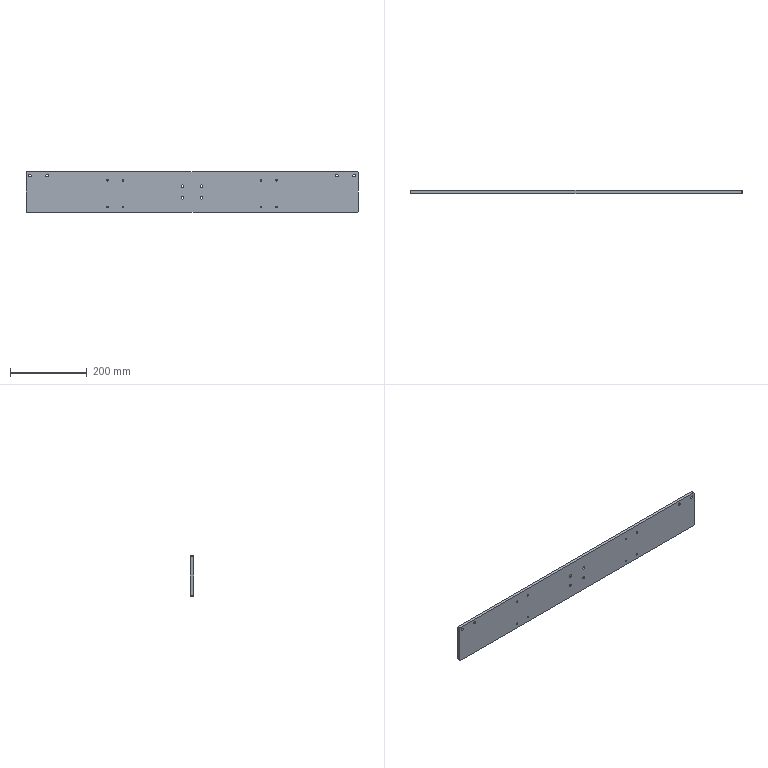Part | SolidWorks | features HoleWzd 3, Chamfer 1, Extrusion 1 | 1 solid | 42 faces | box 865 x 8 x 105 mm | volume 723256 mm3 | cylinder 32 | plane 10 | commonest cylinder face diameters 4.2 x16 6.8 x8 7 x8
STEP:
#1=CARTESIAN_POINT('',(422.5,-4.,39.1));
#2=VERTEX_POINT('',#1);
#3=CARTESIAN_POINT('',(422.5,-4.,45.9));
#4=VERTEX_POINT('',#3);
#5=CARTESIAN_POINT('',(422.5,-4.,42.5));
#6=DIRECTION('',(0.,1.,0.));
#7=DIRECTION('',(0.,0.,1.));
#8=AXIS2_PLACEMENT_3D('',#5,#6,#7);
#9=CIRCLE('',#8,3.4);
#10=EDGE_CURVE('',#2,#4,#9,.T.);
#11=ORIENTED_EDGE('',*,*,#10,.F.);
#12=CARTESIAN_POINT('',(422.5,4.,39.1));
#13=VERTEX_POINT('',#12);
#14=CARTESIAN_POINT('',(422.5,4.,39.1));
#15=DIRECTION('',(0.,1.,0.));
#16=VECTOR('',#15,1000.);
#17=LINE('',#14,#16);
#18=EDGE_CURVE('',#2,#13,#17,.T.);
#19=ORIENTED_EDGE('',*,*,#18,.T.);
#20=CARTESIAN_POINT('',(422.5,4.,45.9));
#21=VERTEX_POINT('',#20);
#22=CARTESIAN_POINT('',(422.5,4.,42.5));
#23=DIRECTION('',(0.,1.,0.));
#24=DIRECTION('',(0.,0.,1.));
#25=AXIS2_PLACEMENT_3D('',#22,#23,#24);
#26=CIRCLE('',#25,3.4);
#27=EDGE_CURVE('',#13,#21,#26,.T.);
#28=ORIENTED_EDGE('',*,*,#27,.T.);
#29=CARTESIAN_POINT('',(422.5,4.,45.9));
#30=DIRECTION('',(0.,1.,0.));
#31=VECTOR('',#30,1000.);
#32=LINE('',#29,#31);
#33=EDGE_CURVE('',#4,#21,#32,.T.);
#34=ORIENTED_EDGE('',*,*,#33,.F.);
#35=EDGE_LOOP('',(#11,#19,#28,#34));
#36=FACE_OUTER_BOUND('',#35,.T.);
#37=CARTESIAN_POINT('',(422.5,4.,42.5));
#38=DIRECTION('',(0.,1.,0.));
#39=DIRECTION('',(0.,0.,1.));
#40=AXIS2_PLACEMENT_3D('',#37,#38,#39);
#41=CYLINDRICAL_SURFACE('',#40,3.4);
#42=ADVANCED_FACE('',(#36),#41,.F.);
#43=CARTESIAN_POINT('',(377.5,-4.,39.1));
#44=VERTEX_POINT('',#43);
#45=CARTESIAN_POINT('',(377.5,-4.,45.9));
#46=VERTEX_POINT('',#45);
#47=CARTESIAN_POINT('',(377.5,-4.,42.5));
#48=DIRECTION('',(0.,1.,0.));
#49=DIRECTION('',(0.,0.,1.));
#50=AXIS2_PLACEMENT_3D('',#47,#48,#49);
#51=CIRCLE('',#50,3.4);
#52=EDGE_CURVE('',#44,#46,#51,.T.);
#53=ORIENTED_EDGE('',*,*,#52,.F.);
#54=CARTESIAN_POINT('',(377.5,4.,39.1));
#55=VERTEX_POINT('',#54);
#56=CARTESIAN_POINT('',(377.5,4.,39.1));
#57=DIRECTION('',(0.,1.,0.));
#58=VECTOR('',#57,1000.);
#59=LINE('',#56,#58);
#60=EDGE_CURVE('',#44,#55,#59,.T.);
#61=ORIENTED_EDGE('',*,*,#60,.T.);
#62=CARTESIAN_POINT('',(377.5,4.,45.9));
#63=VERTEX_POINT('',#62);
#64=CARTESIAN_POINT('',(377.5,4.,42.5));
#65=DIRECTION('',(0.,1.,0.));
#66=DIRECTION('',(0.,0.,1.));
#67=AXIS2_PLACEMENT_3D('',#64,#65,#66);
#68=CIRCLE('',#67,3.4);
#69=EDGE_CURVE('',#55,#63,#68,.T.);
#70=ORIENTED_EDGE('',*,*,#69,.T.);
#71=CARTESIAN_POINT('',(377.5,4.,45.9));
#72=DIRECTION('',(0.,1.,0.));
#73=VECTOR('',#72,1000.);
#74=LINE('',#71,#73);
#75=EDGE_CURVE('',#46,#63,#74,.T.);
#76=ORIENTED_EDGE('',*,*,#75,.F.);
#77=EDGE_LOOP('',(#53,#61,#70,#76));
#78=FACE_OUTER_BOUND('',#77,.T.);
#79=CARTESIAN_POINT('',(377.5,4.,42.5));
#80=DIRECTION('',(0.,1.,0.));
#81=DIRECTION('',(0.,0.,1.));
#82=AXIS2_PLACEMENT_3D('',#79,#80,#81);
#83=CYLINDRICAL_SURFACE('',#82,3.4);
#84=ADVANCED_FACE('',(#78),#83,.F.);
#85=CARTESIAN_POINT('',(-377.5,-4.,39.1));
#86=VERTEX_POINT('',#85);
#87=CARTESIAN_POINT('',(-377.5,-4.,45.9));
#88=VERTEX_POINT('',#87);
#89=CARTESIAN_POINT('',(-377.5,-4.,42.5));
#90=DIRECTION('',(0.,1.,0.));
#91=DIRECTION('',(0.,0.,1.));
#92=AXIS2_PLACEMENT_3D('',#89,#90,#91);
#93=CIRCLE('',#92,3.4);
#94=EDGE_CURVE('',#86,#88,#93,.T.);
#95=ORIENTED_EDGE('',*,*,#94,.F.);
#96=CARTESIAN_POINT('',(-377.5,4.,39.1));
#97=VERTEX_POINT('',#96);
#98=CARTESIAN_POINT('',(-377.5,4.,39.1));
#99=DIRECTION('',(0.,1.,0.));
#100=VECTOR('',#99,1000.);
#101=LINE('',#98,#100);
#102=EDGE_CURVE('',#86,#97,#101,.T.);
#103=ORIENTED_EDGE('',*,*,#102,.T.);
#104=CARTESIAN_POINT('',(-377.5,4.,45.9));
#105=VERTEX_POINT('',#104);
#106=CARTESIAN_POINT('',(-377.5,4.,42.5));
#107=DIRECTION('',(0.,1.,0.));
#108=DIRECTION('',(0.,0.,1.));
#109=AXIS2_PLACEMENT_3D('',#106,#107,#108);
#110=CIRCLE('',#109,3.4);
#111=EDGE_CURVE('',#97,#105,#110,.T.);
#112=ORIENTED_EDGE('',*,*,#111,.T.);
#113=CARTESIAN_POINT('',(-377.5,4.,45.9));
#114=DIRECTION('',(0.,1.,0.));
#115=VECTOR('',#114,1000.);
#116=LINE('',#113,#115);
#117=EDGE_CURVE('',#88,#105,#116,.T.);
#118=ORIENTED_EDGE('',*,*,#117,.F.);
#119=EDGE_LOOP('',(#95,#103,#112,#118));
#120=FACE_OUTER_BOUND('',#119,.T.);
#121=CARTESIAN_POINT('',(-377.5,4.,42.5));
#122=DIRECTION('',(0.,1.,0.));
#123=DIRECTION('',(0.,0.,1.));
#124=AXIS2_PLACEMENT_3D('',#121,#122,#123);
#125=CYLINDRICAL_SURFACE('',#124,3.4);
#126=ADVANCED_FACE('',(#120),#125,.F.);
#127=CARTESIAN_POINT('',(-422.5,-4.,39.1));
#128=VERTEX_POINT('',#127);
#129=CARTESIAN_POINT('',(-422.5,-4.,45.9));
#130=VERTEX_POINT('',#129);
#131=CARTESIAN_POINT('',(-422.5,-4.,42.5));
#132=DIRECTION('',(0.,1.,0.));
#133=DIRECTION('',(0.,0.,1.));
#134=AXIS2_PLACEMENT_3D('',#131,#132,#133);
#135=CIRCLE('',#134,3.4);
#136=EDGE_CURVE('',#128,#130,#135,.T.);
#137=ORIENTED_EDGE('',*,*,#136,.F.);
#138=CARTESIAN_POINT('',(-422.5,4.,39.1));
#139=VERTEX_POINT('',#138);
#140=CARTESIAN_POINT('',(-422.5,4.,39.1));
#141=DIRECTION('',(0.,1.,0.));
#142=VECTOR('',#141,1000.);
#143=LINE('',#140,#142);
#144=EDGE_CURVE('',#128,#139,#143,.T.);
#145=ORIENTED_EDGE('',*,*,#144,.T.);
#146=CARTESIAN_POINT('',(-422.5,4.,45.9));
#147=VERTEX_POINT('',#146);
#148=CARTESIAN_POINT('',(-422.5,4.,42.5));
#149=DIRECTION('',(0.,1.,0.));
#150=DIRECTION('',(0.,0.,1.));
#151=AXIS2_PLACEMENT_3D('',#148,#149,#150);
#152=CIRCLE('',#151,3.4);
#153=EDGE_CURVE('',#139,#147,#152,.T.);
#154=ORIENTED_EDGE('',*,*,#153,.T.);
#155=CARTESIAN_POINT('',(-422.5,4.,45.9));
#156=DIRECTION('',(0.,1.,0.));
#157=VECTOR('',#156,1000.);
#158=LINE('',#155,#157);
#159=EDGE_CURVE('',#130,#147,#158,.T.);
#160=ORIENTED_EDGE('',*,*,#159,.F.);
#161=EDGE_LOOP('',(#137,#145,#154,#160));
#162=FACE_OUTER_BOUND('',#161,.T.);
#163=CARTESIAN_POINT('',(-422.5,4.,42.5));
#164=DIRECTION('',(0.,1.,0.));
#165=DIRECTION('',(0.,0.,1.));
#166=AXIS2_PLACEMENT_3D('',#163,#164,#165);
#167=CYLINDRICAL_SURFACE('',#166,3.4);
#168=ADVANCED_FACE('',(#162),#167,.F.);
#169=CARTESIAN_POINT('',(25.,-4.,11.5));
#170=VERTEX_POINT('',#169);
#171=CARTESIAN_POINT('',(25.,-4.,18.5));
#172=VERTEX_POINT('',#171);
#173=CARTESIAN_POINT('',(25.,-4.,15.));
#174=DIRECTION('',(0.,1.,0.));
#175=DIRECTION('',(0.,0.,1.));
#176=AXIS2_PLACEMENT_3D('',#173,#174,#175);
#177=CIRCLE('',#176,3.5);
#178=EDGE_CURVE('',#170,#172,#177,.T.);
#179=ORIENTED_EDGE('',*,*,#178,.F.);
#180=CARTESIAN_POINT('',(25.,4.,11.5));
#181=VERTEX_POINT('',#180);
#182=CARTESIAN_POINT('',(25.,4.,11.5));
#183=DIRECTION('',(0.,1.,0.));
#184=VECTOR('',#183,1000.);
#185=LINE('',#182,#184);
#186=EDGE_CURVE('',#170,#181,#185,.T.);
#187=ORIENTED_EDGE('',*,*,#186,.T.);
#188=CARTESIAN_POINT('',(25.,4.,18.5));
#189=VERTEX_POINT('',#188);
#190=CARTESIAN_POINT('',(25.,4.,15.));
#191=DIRECTION('',(0.,1.,0.));
#192=DIRECTION('',(0.,0.,1.));
#193=AXIS2_PLACEMENT_3D('',#190,#191,#192);
#194=CIRCLE('',#193,3.5);
#195=EDGE_CURVE('',#181,#189,#194,.T.);
#196=ORIENTED_EDGE('',*,*,#195,.T.);
#197=CARTESIAN_POINT('',(25.,4.,18.5));
#198=DIRECTION('',(0.,1.,0.));
#199=VECTOR('',#198,1000.);
#200=LINE('',#197,#199);
#201=EDGE_CURVE('',#172,#189,#200,.T.);
#202=ORIENTED_EDGE('',*,*,#201,.F.);
#203=EDGE_LOOP('',(#179,#187,#196,#202));
#204=FACE_OUTER_BOUND('',#203,.T.);
#205=CARTESIAN_POINT('',(25.,4.,15.));
#206=DIRECTION('',(0.,1.,0.));
#207=DIRECTION('',(0.,0.,1.));
#208=AXIS2_PLACEMENT_3D('',#205,#206,#207);
#209=CYLINDRICAL_SURFACE('',#208,3.5);
#210=ADVANCED_FACE('',(#204),#209,.F.);
#211=CARTESIAN_POINT('',(25.,-4.,-18.5));
#212=VERTEX_POINT('',#211);
#213=CARTESIAN_POINT('',(25.,-4.,-11.5));
#214=VERTEX_POINT('',#213);
#215=CARTESIAN_POINT('',(25.,-4.,-15.));
#216=DIRECTION('',(0.,1.,0.));
#217=DIRECTION('',(0.,0.,1.));
#218=AXIS2_PLACEMENT_3D('',#215,#216,#217);
#219=CIRCLE('',#218,3.5);
#220=EDGE_CURVE('',#212,#214,#219,.T.);
#221=ORIENTED_EDGE('',*,*,#220,.F.);
#222=CARTESIAN_POINT('',(25.,4.,-18.5));
#223=VERTEX_POINT('',#222);
#224=CARTESIAN_POINT('',(25.,4.,-18.5));
#225=DIRECTION('',(0.,1.,0.));
#226=VECTOR('',#225,1000.);
#227=LINE('',#224,#226);
#228=EDGE_CURVE('',#212,#223,#227,.T.);
#229=ORIENTED_EDGE('',*,*,#228,.T.);
#230=CARTESIAN_POINT('',(25.,4.,-11.5));
#231=VERTEX_POINT('',#230);
#232=CARTESIAN_POINT('',(25.,4.,-15.));
#233=DIRECTION('',(0.,1.,0.));
#234=DIRECTION('',(0.,0.,1.));
#235=AXIS2_PLACEMENT_3D('',#232,#233,#234);
#236=CIRCLE('',#235,3.5);
#237=EDGE_CURVE('',#223,#231,#236,.T.);
#238=ORIENTED_EDGE('',*,*,#237,.T.);
#239=CARTESIAN_POINT('',(25.,4.,-11.5));
#240=DIRECTION('',(0.,1.,0.));
#241=VECTOR('',#240,1000.);
#242=LINE('',#239,#241);
#243=EDGE_CURVE('',#214,#231,#242,.T.);
#244=ORIENTED_EDGE('',*,*,#243,.F.);
#245=EDGE_LOOP('',(#221,#229,#238,#244));
#246=FACE_OUTER_BOUND('',#245,.T.);
#247=CARTESIAN_POINT('',(25.,4.,-15.));
#248=DIRECTION('',(0.,1.,0.));
#249=DIRECTION('',(0.,0.,1.));
#250=AXIS2_PLACEMENT_3D('',#247,#248,#249);
#251=CYLINDRICAL_SURFACE('',#250,3.5);
#252=ADVANCED_FACE('',(#246),#251,.F.);
#253=CARTESIAN_POINT('',(-25.,-4.,-18.5));
#254=VERTEX_POINT('',#253);
#255=CARTESIAN_POINT('',(-25.,-4.,-11.5));
#256=VERTEX_POINT('',#255);
#257=CARTESIAN_POINT('',(-25.,-4.,-15.));
#258=DIRECTION('',(0.,1.,0.));
#259=DIRECTION('',(0.,0.,1.));
#260=AXIS2_PLACEMENT_3D('',#257,#258,#259);
#261=CIRCLE('',#260,3.5);
#262=EDGE_CURVE('',#254,#256,#261,.T.);
#263=ORIENTED_EDGE('',*,*,#262,.F.);
#264=CARTESIAN_POINT('',(-25.,4.,-18.5));
#265=VERTEX_POINT('',#264);
#266=CARTESIAN_POINT('',(-25.,4.,-18.5));
#267=DIRECTION('',(0.,1.,0.));
#268=VECTOR('',#267,1000.);
#269=LINE('',#266,#268);
#270=EDGE_CURVE('',#254,#265,#269,.T.);
#271=ORIENTED_EDGE('',*,*,#270,.T.);
#272=CARTESIAN_POINT('',(-25.,4.,-11.5));
#273=VERTEX_POINT('',#272);
#274=CARTESIAN_POINT('',(-25.,4.,-15.));
#275=DIRECTION('',(0.,1.,0.));
#276=DIRECTION('',(0.,0.,1.));
#277=AXIS2_PLACEMENT_3D('',#274,#275,#276);
#278=CIRCLE('',#277,3.5);
#279=EDGE_CURVE('',#265,#273,#278,.T.);
#280=ORIENTED_EDGE('',*,*,#279,.T.);
#281=CARTESIAN_POINT('',(-25.,4.,-11.5));
#282=DIRECTION('',(0.,1.,0.));
#283=VECTOR('',#282,1000.);
#284=LINE('',#281,#283);
#285=EDGE_CURVE('',#256,#273,#284,.T.);
#286=ORIENTED_EDGE('',*,*,#285,.F.);
#287=EDGE_LOOP('',(#263,#271,#280,#286));
#288=FACE_OUTER_BOUND('',#287,.T.);
#289=CARTESIAN_POINT('',(-25.,4.,-15.));
#290=DIRECTION('',(0.,1.,0.));
#291=DIRECTION('',(0.,0.,1.));
#292=AXIS2_PLACEMENT_3D('',#289,#290,#291);
#293=CYLINDRICAL_SURFACE('',#292,3.5);
#294=ADVANCED_FACE('',(#288),#293,.F.);
#295=CARTESIAN_POINT('',(-25.,-4.,11.5));
#296=VERTEX_POINT('',#295);
#297=CARTESIAN_POINT('',(-25.,-4.,18.5));
#298=VERTEX_POINT('',#297);
#299=CARTESIAN_POINT('',(-25.,-4.,15.));
#300=DIRECTION('',(0.,1.,0.));
#301=DIRECTION('',(0.,0.,1.));
#302=AXIS2_PLACEMENT_3D('',#299,#300,#301);
#303=CIRCLE('',#302,3.5);
#304=EDGE_CURVE('',#296,#298,#303,.T.);
#305=ORIENTED_EDGE('',*,*,#304,.F.);
#306=CARTESIAN_POINT('',(-25.,4.,11.5));
#307=VERTEX_POINT('',#306);
#308=CARTESIAN_POINT('',(-25.,4.,11.5));
#309=DIRECTION('',(0.,1.,0.));
#310=VECTOR('',#309,1000.);
#311=LINE('',#308,#310);
#312=EDGE_CURVE('',#296,#307,#311,.T.);
#313=ORIENTED_EDGE('',*,*,#312,.T.);
#314=CARTESIAN_POINT('',(-25.,4.,18.5));
#315=VERTEX_POINT('',#314);
#316=CARTESIAN_POINT('',(-25.,4.,15.));
#317=DIRECTION('',(0.,1.,0.));
#318=DIRECTION('',(0.,0.,1.));
#319=AXIS2_PLACEMENT_3D('',#316,#317,#318);
#320=CIRCLE('',#319,3.5);
#321=EDGE_CURVE('',#307,#315,#320,.T.);
#322=ORIENTED_EDGE('',*,*,#321,.T.);
#323=CARTESIAN_POINT('',(-25.,4.,18.5));
#324=DIRECTION('',(0.,1.,0.));
#325=VECTOR('',#324,1000.);
#326=LINE('',#323,#325);
#327=EDGE_CURVE('',#298,#315,#326,.T.);
#328=ORIENTED_EDGE('',*,*,#327,.F.);
#329=EDGE_LOOP('',(#305,#313,#322,#328));
#330=FACE_OUTER_BOUND('',#329,.T.);
#331=CARTESIAN_POINT('',(-25.,4.,15.));
#332=DIRECTION('',(0.,1.,0.));
#333=DIRECTION('',(0.,0.,1.));
#334=AXIS2_PLACEMENT_3D('',#331,#332,#333);
#335=CYLINDRICAL_SURFACE('',#334,3.5);
#336=ADVANCED_FACE('',(#330),#335,.F.);
#337=CARTESIAN_POINT('',(-220.,-4.,-41.6));
#338=VERTEX_POINT('',#337);
#339=CARTESIAN_POINT('',(-220.,-4.,-37.4));
#340=VERTEX_POINT('',#339);
#341=CARTESIAN_POINT('',(-220.,-4.,-39.5));
#342=DIRECTION('',(0.,1.,0.));
#343=DIRECTION('',(0.,0.,1.));
#344=AXIS2_PLACEMENT_3D('',#341,#342,#343);
#345=CIRCLE('',#344,2.1);
#346=EDGE_CURVE('',#338,#340,#345,.T.);
#347=ORIENTED_EDGE('',*,*,#346,.F.);
#348=CARTESIAN_POINT('',(-220.,4.,-41.6));
#349=VERTEX_POINT('',#348);
#350=CARTESIAN_POINT('',(-220.,4.,-41.6));
#351=DIRECTION('',(0.,1.,0.));
#352=VECTOR('',#351,1000.);
#353=LINE('',#350,#352);
#354=EDGE_CURVE('',#338,#349,#353,.T.);
#355=ORIENTED_EDGE('',*,*,#354,.T.);
#356=CARTESIAN_POINT('',(-220.,4.,-37.4));
#357=VERTEX_POINT('',#356);
#358=CARTESIAN_POINT('',(-220.,4.,-39.5));
#359=DIRECTION('',(0.,1.,0.));
#360=DIRECTION('',(0.,0.,1.));
#361=AXIS2_PLACEMENT_3D('',#358,#359,#360);
#362=CIRCLE('',#361,2.1);
#363=EDGE_CURVE('',#349,#357,#362,.T.);
#364=ORIENTED_EDGE('',*,*,#363,.T.);
#365=CARTESIAN_POINT('',(-220.,4.,-37.4));
#366=DIRECTION('',(0.,1.,0.));
#367=VECTOR('',#366,1000.);
#368=LINE('',#365,#367);
#369=EDGE_CURVE('',#340,#357,#368,.T.);
#370=ORIENTED_EDGE('',*,*,#369,.F.);
#371=EDGE_LOOP('',(#347,#355,#364,#370));
#372=FACE_OUTER_BOUND('',#371,.T.);
#373=CARTESIAN_POINT('',(-220.,4.,-39.5));
#374=DIRECTION('',(0.,1.,0.));
#375=DIRECTION('',(0.,0.,1.));
#376=AXIS2_PLACEMENT_3D('',#373,#374,#375);
#377=CYLINDRICAL_SURFACE('',#376,2.1);
#378=ADVANCED_FACE('',(#372),#377,.F.);
#379=CARTESIAN_POINT('',(-180.,-4.,-41.6));
#380=VERTEX_POINT('',#379);
#381=CARTESIAN_POINT('',(-180.,-4.,-37.4));
#382=VERTEX_POINT('',#381);
#383=CARTESIAN_POINT('',(-180.,-4.,-39.5));
#384=DIRECTION('',(0.,1.,0.));
#385=DIRECTION('',(0.,0.,1.));
#386=AXIS2_PLACEMENT_3D('',#383,#384,#385);
#387=CIRCLE('',#386,2.1);
#388=EDGE_CURVE('',#380,#382,#387,.T.);
#389=ORIENTED_EDGE('',*,*,#388,.F.);
#390=CARTESIAN_POINT('',(-180.,4.,-41.6));
#391=VERTEX_POINT('',#390);
#392=CARTESIAN_POINT('',(-180.,4.,-41.6));
#393=DIRECTION('',(0.,1.,0.));
#394=VECTOR('',#393,1000.);
#395=LINE('',#392,#394);
#396=EDGE_CURVE('',#380,#391,#395,.T.);
#397=ORIENTED_EDGE('',*,*,#396,.T.);
#398=CARTESIAN_POINT('',(-180.,4.,-37.4));
#399=VERTEX_POINT('',#398);
#400=CARTESIAN_POINT('',(-180.,4.,-39.5));
#401=DIRECTION('',(0.,1.,0.));
#402=DIRECTION('',(0.,0.,1.));
#403=AXIS2_PLACEMENT_3D('',#400,#401,#402);
#404=CIRCLE('',#403,2.1);
#405=EDGE_CURVE('',#391,#399,#404,.T.);
#406=ORIENTED_EDGE('',*,*,#405,.T.);
#407=CARTESIAN_POINT('',(-180.,4.,-37.4));
#408=DIRECTION('',(0.,1.,0.));
#409=VECTOR('',#408,1000.);
#410=LINE('',#407,#409);
#411=EDGE_CURVE('',#382,#399,#410,.T.);
#412=ORIENTED_EDGE('',*,*,#411,.F.);
#413=EDGE_LOOP('',(#389,#397,#406,#412));
#414=FACE_OUTER_BOUND('',#413,.T.);
#415=CARTESIAN_POINT('',(-180.,4.,-39.5));
#416=DIRECTION('',(0.,1.,0.));
#417=DIRECTION('',(0.,0.,1.));
#418=AXIS2_PLACEMENT_3D('',#415,#416,#417);
#419=CYLINDRICAL_SURFACE('',#418,2.1);
#420=ADVANCED_FACE('',(#414),#419,.F.);
#421=CARTESIAN_POINT('',(-180.,-4.,28.4));
#422=VERTEX_POINT('',#421);
#423=CARTESIAN_POINT('',(-180.,-4.,32.6));
#424=VERTEX_POINT('',#423);
#425=CARTESIAN_POINT('',(-180.,-4.,30.5));
#426=DIRECTION('',(0.,1.,0.));
#427=DIRECTION('',(0.,0.,1.));
#428=AXIS2_PLACEMENT_3D('',#425,#426,#427);
#429=CIRCLE('',#428,2.1);
#430=EDGE_CURVE('',#422,#424,#429,.T.);
#431=ORIENTED_EDGE('',*,*,#430,.F.);
#432=CARTESIAN_POINT('',(-180.,4.,28.4));
#433=VERTEX_POINT('',#432);
#434=CARTESIAN_POINT('',(-180.,4.,28.4));
#435=DIRECTION('',(0.,1.,0.));
#436=VECTOR('',#435,1000.);
#437=LINE('',#434,#436);
#438=EDGE_CURVE('',#422,#433,#437,.T.);
#439=ORIENTED_EDGE('',*,*,#438,.T.);
#440=CARTESIAN_POINT('',(-180.,4.,32.6));
#441=VERTEX_POINT('',#440);
#442=CARTESIAN_POINT('',(-180.,4.,30.5));
#443=DIRECTION('',(0.,1.,0.));
#444=DIRECTION('',(0.,0.,1.));
#445=AXIS2_PLACEMENT_3D('',#442,#443,#444);
#446=CIRCLE('',#445,2.1);
#447=EDGE_CURVE('',#433,#441,#446,.T.);
#448=ORIENTED_EDGE('',*,*,#447,.T.);
#449=CARTESIAN_POINT('',(-180.,4.,32.6));
#450=DIRECTION('',(0.,1.,0.));
#451=VECTOR('',#450,1000.);
#452=LINE('',#449,#451);
#453=EDGE_CURVE('',#424,#441,#452,.T.);
#454=ORIENTED_EDGE('',*,*,#453,.F.);
#455=EDGE_LOOP('',(#431,#439,#448,#454));
#456=FACE_OUTER_BOUND('',#455,.T.);
#457=CARTESIAN_POINT('',(-180.,4.,30.5));
#458=DIRECTION('',(0.,1.,0.));
#459=DIRECTION('',(0.,0.,1.));
#460=AXIS2_PLACEMENT_3D('',#457,#458,#459);
#461=CYLINDRICAL_SURFACE('',#460,2.1);
#462=ADVANCED_FACE('',(#456),#461,.F.);
#463=CARTESIAN_POINT('',(-220.,-4.,28.4));
#464=VERTEX_POINT('',#463);
#465=CARTESIAN_POINT('',(-220.,-4.,32.6));
#466=VERTEX_POINT('',#465);
#467=CARTESIAN_POINT('',(-220.,-4.,30.5));
#468=DIRECTION('',(0.,1.,0.));
#469=DIRECTION('',(0.,0.,1.));
#470=AXIS2_PLACEMENT_3D('',#467,#468,#469);
#471=CIRCLE('',#470,2.1);
#472=EDGE_CURVE('',#464,#466,#471,.T.);
#473=ORIENTED_EDGE('',*,*,#472,.F.);
#474=CARTESIAN_POINT('',(-220.,4.,28.4));
#475=VERTEX_POINT('',#474);
#476=CARTESIAN_POINT('',(-220.,4.,28.4));
#477=DIRECTION('',(0.,1.,0.));
#478=VECTOR('',#477,1000.);
#479=LINE('',#476,#478);
#480=EDGE_CURVE('',#464,#475,#479,.T.);
#481=ORIENTED_EDGE('',*,*,#480,.T.);
#482=CARTESIAN_POINT('',(-220.,4.,32.6));
#483=VERTEX_POINT('',#482);
#484=CARTESIAN_POINT('',(-220.,4.,30.5));
#485=DIRECTION('',(0.,1.,0.));
#486=DIRECTION('',(0.,0.,1.));
#487=AXIS2_PLACEMENT_3D('',#484,#485,#486);
#488=CIRCLE('',#487,2.1);
#489=EDGE_CURVE('',#475,#483,#488,.T.);
#490=ORIENTED_EDGE('',*,*,#489,.T.);
#491=CARTESIAN_POINT('',(-220.,4.,32.6));
#492=DIRECTION('',(0.,1.,0.));
#493=VECTOR('',#492,1000.);
#494=LINE('',#491,#493);
#495=EDGE_CURVE('',#466,#483,#494,.T.);
#496=ORIENTED_EDGE('',*,*,#495,.F.);
#497=EDGE_LOOP('',(#473,#481,#490,#496));
#498=FACE_OUTER_BOUND('',#497,.T.);
#499=CARTESIAN_POINT('',(-220.,4.,30.5));
#500=DIRECTION('',(0.,1.,0.));
#501=DIRECTION('',(0.,0.,1.));
#502=AXIS2_PLACEMENT_3D('',#499,#500,#501);
#503=CYLINDRICAL_SURFACE('',#502,2.1);
#504=ADVANCED_FACE('',(#498),#503,.F.);
#505=CARTESIAN_POINT('',(220.,-4.,28.4));
#506=VERTEX_POINT('',#505);
#507=CARTESIAN_POINT('',(220.,-4.,32.6));
#508=VERTEX_POINT('',#507);
#509=CARTESIAN_POINT('',(220.,-4.,30.5));
#510=DIRECTION('',(0.,1.,0.));
#511=DIRECTION('',(0.,0.,1.));
#512=AXIS2_PLACEMENT_3D('',#509,#510,#511);
#513=CIRCLE('',#512,2.1);
#514=EDGE_CURVE('',#506,#508,#513,.T.);
#515=ORIENTED_EDGE('',*,*,#514,.F.);
#516=CARTESIAN_POINT('',(220.,4.,28.4));
#517=VERTEX_POINT('',#516);
#518=CARTESIAN_POINT('',(220.,4.,28.4));
#519=DIRECTION('',(0.,1.,0.));
#520=VECTOR('',#519,1000.);
#521=LINE('',#518,#520);
#522=EDGE_CURVE('',#506,#517,#521,.T.);
#523=ORIENTED_EDGE('',*,*,#522,.T.);
#524=CARTESIAN_POINT('',(220.,4.,32.6));
#525=VERTEX_POINT('',#524);
#526=CARTESIAN_POINT('',(220.,4.,30.5));
#527=DIRECTION('',(0.,1.,0.));
#528=DIRECTION('',(0.,0.,1.));
#529=AXIS2_PLACEMENT_3D('',#526,#527,#528);
#530=CIRCLE('',#529,2.1);
#531=EDGE_CURVE('',#517,#525,#530,.T.);
#532=ORIENTED_EDGE('',*,*,#531,.T.);
#533=CARTESIAN_POINT('',(220.,4.,32.6));
#534=DIRECTION('',(0.,1.,0.));
#535=VECTOR('',#534,1000.);
#536=LINE('',#533,#535);
#537=EDGE_CURVE('',#508,#525,#536,.T.);
#538=ORIENTED_EDGE('',*,*,#537,.F.);
#539=EDGE_LOOP('',(#515,#523,#532,#538));
#540=FACE_OUTER_BOUND('',#539,.T.);
#541=CARTESIAN_POINT('',(220.,4.,30.5));
#542=DIRECTION('',(0.,1.,0.));
#543=DIRECTION('',(0.,0.,1.));
#544=AXIS2_PLACEMENT_3D('',#541,#542,#543);
#545=CYLINDRICAL_SURFACE('',#544,2.1);
#546=ADVANCED_FACE('',(#540),#545,.F.);
#547=CARTESIAN_POINT('',(180.,-4.,28.4));
#548=VERTEX_POINT('',#547);
#549=CARTESIAN_POINT('',(180.,-4.,32.6));
#550=VERTEX_POINT('',#549);
#551=CARTESIAN_POINT('',(180.,-4.,30.5));
#552=DIRECTION('',(0.,1.,0.));
#553=DIRECTION('',(0.,0.,1.));
#554=AXIS2_PLACEMENT_3D('',#551,#552,#553);
#555=CIRCLE('',#554,2.1);
#556=EDGE_CURVE('',#548,#550,#555,.T.);
#557=ORIENTED_EDGE('',*,*,#556,.F.);
#558=CARTESIAN_POINT('',(180.,4.,28.4));
#559=VERTEX_POINT('',#558);
#560=CARTESIAN_POINT('',(180.,4.,28.4));
#561=DIRECTION('',(0.,1.,0.));
#562=VECTOR('',#561,1000.);
#563=LINE('',#560,#562);
#564=EDGE_CURVE('',#548,#559,#563,.T.);
#565=ORIENTED_EDGE('',*,*,#564,.T.);
#566=CARTESIAN_POINT('',(180.,4.,32.6));
#567=VERTEX_POINT('',#566);
#568=CARTESIAN_POINT('',(180.,4.,30.5));
#569=DIRECTION('',(0.,1.,0.));
#570=DIRECTION('',(0.,0.,1.));
#571=AXIS2_PLACEMENT_3D('',#568,#569,#570);
#572=CIRCLE('',#571,2.1);
#573=EDGE_CURVE('',#559,#567,#572,.T.);
#574=ORIENTED_EDGE('',*,*,#573,.T.);
#575=CARTESIAN_POINT('',(180.,4.,32.6));
#576=DIRECTION('',(0.,1.,0.));
#577=VECTOR('',#576,1000.);
#578=LINE('',#575,#577);
#579=EDGE_CURVE('',#550,#567,#578,.T.);
#580=ORIENTED_EDGE('',*,*,#579,.F.);
#581=EDGE_LOOP('',(#557,#565,#574,#580));
#582=FACE_OUTER_BOUND('',#581,.T.);
#583=CARTESIAN_POINT('',(180.,4.,30.5));
#584=DIRECTION('',(0.,1.,0.));
#585=DIRECTION('',(0.,0.,1.));
#586=AXIS2_PLACEMENT_3D('',#583,#584,#585);
#587=CYLINDRICAL_SURFACE('',#586,2.1);
#588=ADVANCED_FACE('',(#582),#587,.F.);
#589=CARTESIAN_POINT('',(180.,-4.,-41.6));
#590=VERTEX_POINT('',#589);
#591=CARTESIAN_POINT('',(180.,-4.,-37.4));
#592=VERTEX_POINT('',#591);
#593=CARTESIAN_POINT('',(180.,-4.,-39.5));
#594=DIRECTION('',(0.,1.,0.));
#595=DIRECTION('',(0.,0.,1.));
#596=AXIS2_PLACEMENT_3D('',#593,#594,#595);
#597=CIRCLE('',#596,2.1);
#598=EDGE_CURVE('',#590,#592,#597,.T.);
#599=ORIENTED_EDGE('',*,*,#598,.F.);
#600=CARTESIAN_POINT('',(180.,4.,-41.6));
#601=VERTEX_POINT('',#600);
#602=CARTESIAN_POINT('',(180.,4.,-41.6));
#603=DIRECTION('',(0.,1.,0.));
#604=VECTOR('',#603,1000.);
#605=LINE('',#602,#604);
#606=EDGE_CURVE('',#590,#601,#605,.T.);
#607=ORIENTED_EDGE('',*,*,#606,.T.);
#608=CARTESIAN_POINT('',(180.,4.,-37.4));
#609=VERTEX_POINT('',#608);
#610=CARTESIAN_POINT('',(180.,4.,-39.5));
#611=DIRECTION('',(0.,1.,0.));
#612=DIRECTION('',(0.,0.,1.));
#613=AXIS2_PLACEMENT_3D('',#610,#611,#612);
#614=CIRCLE('',#613,2.1);
#615=EDGE_CURVE('',#601,#609,#614,.T.);
#616=ORIENTED_EDGE('',*,*,#615,.T.);
#617=CARTESIAN_POINT('',(180.,4.,-37.4));
#618=DIRECTION('',(0.,1.,0.));
#619=VECTOR('',#618,1000.);
#620=LINE('',#617,#619);
#621=EDGE_CURVE('',#592,#609,#620,.T.);
#622=ORIENTED_EDGE('',*,*,#621,.F.);
#623=EDGE_LOOP('',(#599,#607,#616,#622));
#624=FACE_OUTER_BOUND('',#623,.T.);
#625=CARTESIAN_POINT('',(180.,4.,-39.5));
#626=DIRECTION('',(0.,1.,0.));
#627=DIRECTION('',(0.,0.,1.));
#628=AXIS2_PLACEMENT_3D('',#625,#626,#627);
#629=CYLINDRICAL_SURFACE('',#628,2.1);
#630=ADVANCED_FACE('',(#624),#629,.F.);
#631=CARTESIAN_POINT('',(220.,-4.,-41.6));
#632=VERTEX_POINT('',#631);
#633=CARTESIAN_POINT('',(220.,-4.,-37.4));
#634=VERTEX_POINT('',#633);
#635=CARTESIAN_POINT('',(220.,-4.,-39.5));
#636=DIRECTION('',(0.,1.,0.));
#637=DIRECTION('',(0.,0.,1.));
#638=AXIS2_PLACEMENT_3D('',#635,#636,#637);
#639=CIRCLE('',#638,2.1);
#640=EDGE_CURVE('',#632,#634,#639,.T.);
#641=ORIENTED_EDGE('',*,*,#640,.F.);
#642=CARTESIAN_POINT('',(220.,4.,-41.6));
#643=VERTEX_POINT('',#642);
#644=CARTESIAN_POINT('',(220.,4.,-41.6));
#645=DIRECTION('',(0.,1.,0.));
#646=VECTOR('',#645,1000.);
#647=LINE('',#644,#646);
#648=EDGE_CURVE('',#632,#643,#647,.T.);
#649=ORIENTED_EDGE('',*,*,#648,.T.);
#650=CARTESIAN_POINT('',(220.,4.,-37.4));
#651=VERTEX_POINT('',#650);
#652=CARTESIAN_POINT('',(220.,4.,-39.5));
#653=DIRECTION('',(0.,1.,0.));
#654=DIRECTION('',(0.,0.,1.));
#655=AXIS2_PLACEMENT_3D('',#652,#653,#654);
#656=CIRCLE('',#655,2.1);
#657=EDGE_CURVE('',#643,#651,#656,.T.);
#658=ORIENTED_EDGE('',*,*,#657,.T.);
#659=CARTESIAN_POINT('',(220.,4.,-37.4));
#660=DIRECTION('',(0.,1.,0.));
#661=VECTOR('',#660,1000.);
#662=LINE('',#659,#661);
#663=EDGE_CURVE('',#634,#651,#662,.T.);
#664=ORIENTED_EDGE('',*,*,#663,.F.);
#665=EDGE_LOOP('',(#641,#649,#658,#664));
#666=FACE_OUTER_BOUND('',#665,.T.);
#667=CARTESIAN_POINT('',(220.,4.,-39.5));
#668=DIRECTION('',(0.,1.,0.));
#669=DIRECTION('',(0.,0.,1.));
#670=AXIS2_PLACEMENT_3D('',#667,#668,#669);
#671=CYLINDRICAL_SURFACE('',#670,2.1);
#672=ADVANCED_FACE('',(#666),#671,.F.);
#673=CARTESIAN_POINT('',(432.5,-4.,50.5));
#674=VERTEX_POINT('',#673);
#675=CARTESIAN_POINT('',(432.5,-4.,-50.5));
#676=VERTEX_POINT('',#675);
#677=CARTESIAN_POINT('',(432.5,-4.,52.5));
#678=DIRECTION('',(0.,0.,-1.));
#679=VECTOR('',#678,1000.);
#680=LINE('',#677,#679);
#681=EDGE_CURVE('',#674,#676,#680,.T.);
#682=ORIENTED_EDGE('',*,*,#681,.T.);
#683=CARTESIAN_POINT('',(432.5,4.,-50.5));
#684=VERTEX_POINT('',#683);
#685=CARTESIAN_POINT('',(432.5,4.,-50.5));
#686=DIRECTION('',(0.,1.,0.));
#687=VECTOR('',#686,1000.);
#688=LINE('',#685,#687);
#689=EDGE_CURVE('',#676,#684,#688,.T.);
#690=ORIENTED_EDGE('',*,*,#689,.T.);
#691=CARTESIAN_POINT('',(432.5,4.,50.5));
#692=VERTEX_POINT('',#691);
#693=CARTESIAN_POINT('',(432.5,4.,52.5));
#694=DIRECTION('',(0.,0.,-1.));
#695=VECTOR('',#694,1000.);
#696=LINE('',#693,#695);
#697=EDGE_CURVE('',#692,#684,#696,.T.);
#698=ORIENTED_EDGE('',*,*,#697,.F.);
#699=CARTESIAN_POINT('',(432.5,4.,50.5));
#700=DIRECTION('',(0.,-1.,0.));
#701=VECTOR('',#700,1000.);
#702=LINE('',#699,#701);
#703=EDGE_CURVE('',#692,#674,#702,.T.);
#704=ORIENTED_EDGE('',*,*,#703,.T.);
#705=EDGE_LOOP('',(#682,#690,#698,#704));
#706=FACE_OUTER_BOUND('',#705,.T.);
#707=CARTESIAN_POINT('',(432.5,4.,52.5));
#708=DIRECTION('',(-1.,0.,0.));
#709=DIRECTION('',(0.,0.,1.));
#710=AXIS2_PLACEMENT_3D('',#707,#708,#709);
#711=PLANE('',#710);
#712=ADVANCED_FACE('',(#706),#711,.F.);
#713=CARTESIAN_POINT('',(430.5,4.,-52.5));
#714=VERTEX_POINT('',#713);
#715=CARTESIAN_POINT('',(-430.5,4.,-52.5));
#716=VERTEX_POINT('',#715);
#717=CARTESIAN_POINT('',(-432.5,4.,-52.5));
#718=DIRECTION('',(-1.,0.,0.));
#719=VECTOR('',#718,1000.);
#720=LINE('',#717,#719);
#721=EDGE_CURVE('',#714,#716,#720,.T.);
#722=ORIENTED_EDGE('',*,*,#721,.F.);
#723=CARTESIAN_POINT('',(430.5,-4.,-52.5));
#724=VERTEX_POINT('',#723);
#725=CARTESIAN_POINT('',(430.5,4.,-52.5));
#726=DIRECTION('',(0.,-1.,0.));
#727=VECTOR('',#726,1000.);
#728=LINE('',#725,#727);
#729=EDGE_CURVE('',#714,#724,#728,.T.);
#730=ORIENTED_EDGE('',*,*,#729,.T.);
#731=CARTESIAN_POINT('',(-430.5,-4.,-52.5));
#732=VERTEX_POINT('',#731);
#733=CARTESIAN_POINT('',(-432.5,-4.,-52.5));
#734=DIRECTION('',(-1.,0.,0.));
#735=VECTOR('',#734,1000.);
#736=LINE('',#733,#735);
#737=EDGE_CURVE('',#724,#732,#736,.T.);
#738=ORIENTED_EDGE('',*,*,#737,.T.);
#739=CARTESIAN_POINT('',(-430.5,4.,-52.5));
#740=DIRECTION('',(0.,1.,0.));
#741=VECTOR('',#740,1000.);
#742=LINE('',#739,#741);
#743=EDGE_CURVE('',#732,#716,#742,.T.);
#744=ORIENTED_EDGE('',*,*,#743,.T.);
#745=EDGE_LOOP('',(#722,#730,#738,#744));
#746=FACE_OUTER_BOUND('',#745,.T.);
#747=CARTESIAN_POINT('',(-432.5,4.,-52.5));
#748=DIRECTION('',(0.,0.,1.));
#749=DIRECTION('',(1.,0.,0.));
#750=AXIS2_PLACEMENT_3D('',#747,#748,#749);
#751=PLANE('',#750);
#752=ADVANCED_FACE('',(#746),#751,.F.);
#753=CARTESIAN_POINT('',(-432.5,4.,-50.5));
#754=VERTEX_POINT('',#753);
#755=CARTESIAN_POINT('',(-432.5,4.,50.5));
#756=VERTEX_POINT('',#755);
#757=CARTESIAN_POINT('',(-432.5,4.,52.5));
#758=DIRECTION('',(0.,0.,1.));
#759=VECTOR('',#758,1000.);
#760=LINE('',#757,#759);
#761=EDGE_CURVE('',#754,#756,#760,.T.);
#762=ORIENTED_EDGE('',*,*,#761,.F.);
#763=CARTESIAN_POINT('',(-432.5,-4.,-50.5));
#764=VERTEX_POINT('',#763);
#765=CARTESIAN_POINT('',(-432.5,4.,-50.5));
#766=DIRECTION('',(0.,-1.,0.));
#767=VECTOR('',#766,1000.);
#768=LINE('',#765,#767);
#769=EDGE_CURVE('',#754,#764,#768,.T.);
#770=ORIENTED_EDGE('',*,*,#769,.T.);
#771=CARTESIAN_POINT('',(-432.5,-4.,50.5));
#772=VERTEX_POINT('',#771);
#773=CARTESIAN_POINT('',(-432.5,-4.,52.5));
#774=DIRECTION('',(0.,0.,1.));
#775=VECTOR('',#774,1000.);
#776=LINE('',#773,#775);
#777=EDGE_CURVE('',#764,#772,#776,.T.);
#778=ORIENTED_EDGE('',*,*,#777,.T.);
#779=CARTESIAN_POINT('',(-432.5,4.,50.5));
#780=DIRECTION('',(0.,1.,0.));
#781=VECTOR('',#780,1000.);
#782=LINE('',#779,#781);
#783=EDGE_CURVE('',#772,#756,#782,.T.);
#784=ORIENTED_EDGE('',*,*,#783,.T.);
#785=EDGE_LOOP('',(#762,#770,#778,#784));
#786=FACE_OUTER_BOUND('',#785,.T.);
#787=CARTESIAN_POINT('',(-432.5,4.,52.5));
#788=DIRECTION('',(1.,0.,0.));
#789=DIRECTION('',(0.,0.,-1.));
#790=AXIS2_PLACEMENT_3D('',#787,#788,#789);
#791=PLANE('',#790);
#792=ADVANCED_FACE('',(#786),#791,.F.);
#793=CARTESIAN_POINT('',(-430.5,-4.,52.5));
#794=VERTEX_POINT('',#793);
#795=CARTESIAN_POINT('',(430.5,-4.,52.5));
#796=VERTEX_POINT('',#795);
#797=CARTESIAN_POINT('',(-432.5,-4.,52.5));
#798=DIRECTION('',(1.,0.,0.));
#799=VECTOR('',#798,1000.);
#800=LINE('',#797,#799);
#801=EDGE_CURVE('',#794,#796,#800,.T.);
#802=ORIENTED_EDGE('',*,*,#801,.T.);
#803=CARTESIAN_POINT('',(430.5,4.,52.5));
#804=VERTEX_POINT('',#803);
#805=CARTESIAN_POINT('',(430.5,4.,52.5));
#806=DIRECTION('',(0.,1.,0.));
#807=VECTOR('',#806,1000.);
#808=LINE('',#805,#807);
#809=EDGE_CURVE('',#796,#804,#808,.T.);
#810=ORIENTED_EDGE('',*,*,#809,.T.);
#811=CARTESIAN_POINT('',(-430.5,4.,52.5));
#812=VERTEX_POINT('',#811);
#813=CARTESIAN_POINT('',(-432.5,4.,52.5));
#814=DIRECTION('',(1.,0.,0.));
#815=VECTOR('',#814,1000.);
#816=LINE('',#813,#815);
#817=EDGE_CURVE('',#812,#804,#816,.T.);
#818=ORIENTED_EDGE('',*,*,#817,.F.);
#819=CARTESIAN_POINT('',(-430.5,4.,52.5));
#820=DIRECTION('',(0.,-1.,0.));
#821=VECTOR('',#820,1000.);
#822=LINE('',#819,#821);
#823=EDGE_CURVE('',#812,#794,#822,.T.);
#824=ORIENTED_EDGE('',*,*,#823,.T.);
#825=EDGE_LOOP('',(#802,#810,#818,#824));
#826=FACE_OUTER_BOUND('',#825,.T.);
#827=CARTESIAN_POINT('',(-432.5,4.,52.5));
#828=DIRECTION('',(0.,0.,-1.));
#829=DIRECTION('',(-1.,0.,0.));
#830=AXIS2_PLACEMENT_3D('',#827,#828,#829);
#831=PLANE('',#830);
#832=ADVANCED_FACE('',(#826),#831,.F.);
#833=CARTESIAN_POINT('',(422.5,4.,42.5));
#834=DIRECTION('',(0.,1.,0.));
#835=DIRECTION('',(0.,0.,1.));
#836=AXIS2_PLACEMENT_3D('',#833,#834,#835);
#837=CIRCLE('',#836,3.4);
#838=EDGE_CURVE('',#21,#13,#837,.T.);
#839=ORIENTED_EDGE('',*,*,#838,.F.);
#840=ORIENTED_EDGE('',*,*,#27,.F.);
#841=EDGE_LOOP('',(#839,#840));
#842=FACE_BOUND('',#841,.T.);
#843=CARTESIAN_POINT('',(377.5,4.,42.5));
#844=DIRECTION('',(0.,1.,0.));
#845=DIRECTION('',(0.,0.,1.));
#846=AXIS2_PLACEMENT_3D('',#843,#844,#845);
#847=CIRCLE('',#846,3.4);
#848=EDGE_CURVE('',#63,#55,#847,.T.);
#849=ORIENTED_EDGE('',*,*,#848,.F.);
#850=ORIENTED_EDGE('',*,*,#69,.F.);
#851=EDGE_LOOP('',(#849,#850));
#852=FACE_BOUND('',#851,.T.);
#853=CARTESIAN_POINT('',(-377.5,4.,42.5));
#854=DIRECTION('',(0.,1.,0.));
#855=DIRECTION('',(0.,0.,1.));
#856=AXIS2_PLACEMENT_3D('',#853,#854,#855);
#857=CIRCLE('',#856,3.4);
#858=EDGE_CURVE('',#105,#97,#857,.T.);
#859=ORIENTED_EDGE('',*,*,#858,.F.);
#860=ORIENTED_EDGE('',*,*,#111,.F.);
#861=EDGE_LOOP('',(#859,#860));
#862=FACE_BOUND('',#861,.T.);
#863=CARTESIAN_POINT('',(-422.5,4.,42.5));
#864=DIRECTION('',(0.,1.,0.));
#865=DIRECTION('',(0.,0.,1.));
#866=AXIS2_PLACEMENT_3D('',#863,#864,#865);
#867=CIRCLE('',#866,3.4);
#868=EDGE_CURVE('',#147,#139,#867,.T.);
#869=ORIENTED_EDGE('',*,*,#868,.F.);
#870=ORIENTED_EDGE('',*,*,#153,.F.);
#871=EDGE_LOOP('',(#869,#870));
#872=FACE_BOUND('',#871,.T.);
#873=CARTESIAN_POINT('',(25.,4.,15.));
#874=DIRECTION('',(0.,1.,0.));
#875=DIRECTION('',(0.,0.,1.));
#876=AXIS2_PLACEMENT_3D('',#873,#874,#875);
#877=CIRCLE('',#876,3.5);
#878=EDGE_CURVE('',#189,#181,#877,.T.);
#879=ORIENTED_EDGE('',*,*,#878,.F.);
#880=ORIENTED_EDGE('',*,*,#195,.F.);
#881=EDGE_LOOP('',(#879,#880));
#882=FACE_BOUND('',#881,.T.);
#883=CARTESIAN_POINT('',(25.,4.,-15.));
#884=DIRECTION('',(0.,1.,0.));
#885=DIRECTION('',(0.,0.,1.));
#886=AXIS2_PLACEMENT_3D('',#883,#884,#885);
#887=CIRCLE('',#886,3.5);
#888=EDGE_CURVE('',#231,#223,#887,.T.);
#889=ORIENTED_EDGE('',*,*,#888,.F.);
#890=ORIENTED_EDGE('',*,*,#237,.F.);
#891=EDGE_LOOP('',(#889,#890));
#892=FACE_BOUND('',#891,.T.);
#893=CARTESIAN_POINT('',(-25.,4.,-15.));
#894=DIRECTION('',(0.,1.,0.));
#895=DIRECTION('',(0.,0.,1.));
#896=AXIS2_PLACEMENT_3D('',#893,#894,#895);
#897=CIRCLE('',#896,3.5);
#898=EDGE_CURVE('',#273,#265,#897,.T.);
#899=ORIENTED_EDGE('',*,*,#898,.F.);
#900=ORIENTED_EDGE('',*,*,#279,.F.);
#901=EDGE_LOOP('',(#899,#900));
#902=FACE_BOUND('',#901,.T.);
#903=CARTESIAN_POINT('',(-25.,4.,15.));
#904=DIRECTION('',(0.,1.,0.));
#905=DIRECTION('',(0.,0.,1.));
#906=AXIS2_PLACEMENT_3D('',#903,#904,#905);
#907=CIRCLE('',#906,3.5);
#908=EDGE_CURVE('',#315,#307,#907,.T.);
#909=ORIENTED_EDGE('',*,*,#908,.F.);
#910=ORIENTED_EDGE('',*,*,#321,.F.);
#911=EDGE_LOOP('',(#909,#910));
#912=FACE_BOUND('',#911,.T.);
#913=CARTESIAN_POINT('',(-220.,4.,-39.5));
#914=DIRECTION('',(0.,1.,0.));
#915=DIRECTION('',(0.,0.,1.));
#916=AXIS2_PLACEMENT_3D('',#913,#914,#915);
#917=CIRCLE('',#916,2.1);
#918=EDGE_CURVE('',#357,#349,#917,.T.);
#919=ORIENTED_EDGE('',*,*,#918,.F.);
#920=ORIENTED_EDGE('',*,*,#363,.F.);
#921=EDGE_LOOP('',(#919,#920));
#922=FACE_BOUND('',#921,.T.);
#923=CARTESIAN_POINT('',(-180.,4.,-39.5));
#924=DIRECTION('',(0.,1.,0.));
#925=DIRECTION('',(0.,0.,1.));
#926=AXIS2_PLACEMENT_3D('',#923,#924,#925);
#927=CIRCLE('',#926,2.1);
#928=EDGE_CURVE('',#399,#391,#927,.T.);
#929=ORIENTED_EDGE('',*,*,#928,.F.);
#930=ORIENTED_EDGE('',*,*,#405,.F.);
#931=EDGE_LOOP('',(#929,#930));
#932=FACE_BOUND('',#931,.T.);
#933=CARTESIAN_POINT('',(-180.,4.,30.5));
#934=DIRECTION('',(0.,1.,0.));
#935=DIRECTION('',(0.,0.,1.));
#936=AXIS2_PLACEMENT_3D('',#933,#934,#935);
#937=CIRCLE('',#936,2.1);
#938=EDGE_CURVE('',#441,#433,#937,.T.);
#939=ORIENTED_EDGE('',*,*,#938,.F.);
#940=ORIENTED_EDGE('',*,*,#447,.F.);
#941=EDGE_LOOP('',(#939,#940));
#942=FACE_BOUND('',#941,.T.);
#943=CARTESIAN_POINT('',(-220.,4.,30.5));
#944=DIRECTION('',(0.,1.,0.));
#945=DIRECTION('',(0.,0.,1.));
#946=AXIS2_PLACEMENT_3D('',#943,#944,#945);
#947=CIRCLE('',#946,2.1);
#948=EDGE_CURVE('',#483,#475,#947,.T.);
#949=ORIENTED_EDGE('',*,*,#948,.F.);
#950=ORIENTED_EDGE('',*,*,#489,.F.);
#951=EDGE_LOOP('',(#949,#950));
#952=FACE_BOUND('',#951,.T.);
#953=CARTESIAN_POINT('',(220.,4.,30.5));
#954=DIRECTION('',(0.,1.,0.));
#955=DIRECTION('',(0.,0.,1.));
#956=AXIS2_PLACEMENT_3D('',#953,#954,#955);
#957=CIRCLE('',#956,2.1);
#958=EDGE_CURVE('',#525,#517,#957,.T.);
#959=ORIENTED_EDGE('',*,*,#958,.F.);
#960=ORIENTED_EDGE('',*,*,#531,.F.);
#961=EDGE_LOOP('',(#959,#960));
#962=FACE_BOUND('',#961,.T.);
#963=CARTESIAN_POINT('',(180.,4.,30.5));
#964=DIRECTION('',(0.,1.,0.));
#965=DIRECTION('',(0.,0.,1.));
#966=AXIS2_PLACEMENT_3D('',#963,#964,#965);
#967=CIRCLE('',#966,2.1);
#968=EDGE_CURVE('',#567,#559,#967,.T.);
#969=ORIENTED_EDGE('',*,*,#968,.F.);
#970=ORIENTED_EDGE('',*,*,#573,.F.);
#971=EDGE_LOOP('',(#969,#970));
#972=FACE_BOUND('',#971,.T.);
#973=CARTESIAN_POINT('',(180.,4.,-39.5));
#974=DIRECTION('',(0.,1.,0.));
#975=DIRECTION('',(0.,0.,1.));
#976=AXIS2_PLACEMENT_3D('',#973,#974,#975);
#977=CIRCLE('',#976,2.1);
#978=EDGE_CURVE('',#609,#601,#977,.T.);
#979=ORIENTED_EDGE('',*,*,#978,.F.);
#980=ORIENTED_EDGE('',*,*,#615,.F.);
#981=EDGE_LOOP('',(#979,#980));
#982=FACE_BOUND('',#981,.T.);
#983=CARTESIAN_POINT('',(220.,4.,-39.5));
#984=DIRECTION('',(0.,1.,0.));
#985=DIRECTION('',(0.,0.,1.));
#986=AXIS2_PLACEMENT_3D('',#983,#984,#985);
#987=CIRCLE('',#986,2.1);
#988=EDGE_CURVE('',#651,#643,#987,.T.);
#989=ORIENTED_EDGE('',*,*,#988,.F.);
#990=ORIENTED_EDGE('',*,*,#657,.F.);
#991=EDGE_LOOP('',(#989,#990));
#992=FACE_BOUND('',#991,.T.);
#993=ORIENTED_EDGE('',*,*,#697,.T.);
#994=CARTESIAN_POINT('',(430.5,4.,-52.5));
#995=DIRECTION('',(-0.7071,0.,-0.7071));
#996=VECTOR('',#995,1000.);
#997=LINE('',#994,#996);
#998=EDGE_CURVE('',#684,#714,#997,.T.);
#999=ORIENTED_EDGE('',*,*,#998,.T.);
#1000=ORIENTED_EDGE('',*,*,#721,.T.);
#1001=CARTESIAN_POINT('',(-432.5,4.,-50.5));
#1002=DIRECTION('',(-0.7071,0.,0.7071));
#1003=VECTOR('',#1002,1000.);
#1004=LINE('',#1001,#1003);
#1005=EDGE_CURVE('',#716,#754,#1004,.T.);
#1006=ORIENTED_EDGE('',*,*,#1005,.T.);
#1007=ORIENTED_EDGE('',*,*,#761,.T.);
#1008=CARTESIAN_POINT('',(-430.5,4.,52.5));
#1009=DIRECTION('',(0.7071,0.,0.7071));
#1010=VECTOR('',#1009,1000.);
#1011=LINE('',#1008,#1010);
#1012=EDGE_CURVE('',#756,#812,#1011,.T.);
#1013=ORIENTED_EDGE('',*,*,#1012,.T.);
#1014=ORIENTED_EDGE('',*,*,#817,.T.);
#1015=CARTESIAN_POINT('',(432.5,4.,50.5));
#1016=DIRECTION('',(0.7071,0.,-0.7071));
#1017=VECTOR('',#1016,1000.);
#1018=LINE('',#1015,#1017);
#1019=EDGE_CURVE('',#804,#692,#1018,.T.);
#1020=ORIENTED_EDGE('',*,*,#1019,.T.);
#1021=EDGE_LOOP('',(#993,#999,#1000,#1006,#1007,#1013,#1014,#1020));
#1022=FACE_OUTER_BOUND('',#1021,.T.);
#1023=CARTESIAN_POINT('',(0.,4.,0.));
#1024=DIRECTION('',(0.,-1.,0.));
#1025=DIRECTION('',(0.,0.,-1.));
#1026=AXIS2_PLACEMENT_3D('',#1023,#1024,#1025);
#1027=PLANE('',#1026);
#1028=ADVANCED_FACE('',(#842,#852,#862,#872,#882,#892,#902,#912,#922,#932,#942,#952,#962,#972,#982,#992,#1022),#1027,.F.);
#1029=CARTESIAN_POINT('',(422.5,-4.,42.5));
#1030=DIRECTION('',(0.,1.,0.));
#1031=DIRECTION('',(0.,0.,1.));
#1032=AXIS2_PLACEMENT_3D('',#1029,#1030,#1031);
#1033=CIRCLE('',#1032,3.4);
#1034=EDGE_CURVE('',#4,#2,#1033,.T.);
#1035=ORIENTED_EDGE('',*,*,#1034,.T.);
#1036=ORIENTED_EDGE('',*,*,#10,.T.);
#1037=EDGE_LOOP('',(#1035,#1036));
#1038=FACE_BOUND('',#1037,.T.);
#1039=CARTESIAN_POINT('',(377.5,-4.,42.5));
#1040=DIRECTION('',(0.,1.,0.));
#1041=DIRECTION('',(0.,0.,1.));
#1042=AXIS2_PLACEMENT_3D('',#1039,#1040,#1041);
#1043=CIRCLE('',#1042,3.4);
#1044=EDGE_CURVE('',#46,#44,#1043,.T.);
#1045=ORIENTED_EDGE('',*,*,#1044,.T.);
#1046=ORIENTED_EDGE('',*,*,#52,.T.);
#1047=EDGE_LOOP('',(#1045,#1046));
#1048=FACE_BOUND('',#1047,.T.);
#1049=CARTESIAN_POINT('',(-377.5,-4.,42.5));
#1050=DIRECTION('',(0.,1.,0.));
#1051=DIRECTION('',(0.,0.,1.));
#1052=AXIS2_PLACEMENT_3D('',#1049,#1050,#1051);
#1053=CIRCLE('',#1052,3.4);
#1054=EDGE_CURVE('',#88,#86,#1053,.T.);
#1055=ORIENTED_EDGE('',*,*,#1054,.T.);
#1056=ORIENTED_EDGE('',*,*,#94,.T.);
#1057=EDGE_LOOP('',(#1055,#1056));
#1058=FACE_BOUND('',#1057,.T.);
#1059=CARTESIAN_POINT('',(-422.5,-4.,42.5));
#1060=DIRECTION('',(0.,1.,0.));
#1061=DIRECTION('',(0.,0.,1.));
#1062=AXIS2_PLACEMENT_3D('',#1059,#1060,#1061);
#1063=CIRCLE('',#1062,3.4);
#1064=EDGE_CURVE('',#130,#128,#1063,.T.);
#1065=ORIENTED_EDGE('',*,*,#1064,.T.);
#1066=ORIENTED_EDGE('',*,*,#136,.T.);
#1067=EDGE_LOOP('',(#1065,#1066));
#1068=FACE_BOUND('',#1067,.T.);
#1069=CARTESIAN_POINT('',(25.,-4.,15.));
#1070=DIRECTION('',(0.,1.,0.));
#1071=DIRECTION('',(0.,0.,1.));
#1072=AXIS2_PLACEMENT_3D('',#1069,#1070,#1071);
#1073=CIRCLE('',#1072,3.5);
#1074=EDGE_CURVE('',#172,#170,#1073,.T.);
#1075=ORIENTED_EDGE('',*,*,#1074,.T.);
#1076=ORIENTED_EDGE('',*,*,#178,.T.);
#1077=EDGE_LOOP('',(#1075,#1076));
#1078=FACE_BOUND('',#1077,.T.);
#1079=CARTESIAN_POINT('',(25.,-4.,-15.));
#1080=DIRECTION('',(0.,1.,0.));
#1081=DIRECTION('',(0.,0.,1.));
#1082=AXIS2_PLACEMENT_3D('',#1079,#1080,#1081);
#1083=CIRCLE('',#1082,3.5);
#1084=EDGE_CURVE('',#214,#212,#1083,.T.);
#1085=ORIENTED_EDGE('',*,*,#1084,.T.);
#1086=ORIENTED_EDGE('',*,*,#220,.T.);
#1087=EDGE_LOOP('',(#1085,#1086));
#1088=FACE_BOUND('',#1087,.T.);
#1089=CARTESIAN_POINT('',(-25.,-4.,-15.));
#1090=DIRECTION('',(0.,1.,0.));
#1091=DIRECTION('',(0.,0.,1.));
#1092=AXIS2_PLACEMENT_3D('',#1089,#1090,#1091);
#1093=CIRCLE('',#1092,3.5);
#1094=EDGE_CURVE('',#256,#254,#1093,.T.);
#1095=ORIENTED_EDGE('',*,*,#1094,.T.);
#1096=ORIENTED_EDGE('',*,*,#262,.T.);
#1097=EDGE_LOOP('',(#1095,#1096));
#1098=FACE_BOUND('',#1097,.T.);
#1099=CARTESIAN_POINT('',(-25.,-4.,15.));
#1100=DIRECTION('',(0.,1.,0.));
#1101=DIRECTION('',(0.,0.,1.));
#1102=AXIS2_PLACEMENT_3D('',#1099,#1100,#1101);
#1103=CIRCLE('',#1102,3.5);
#1104=EDGE_CURVE('',#298,#296,#1103,.T.);
#1105=ORIENTED_EDGE('',*,*,#1104,.T.);
#1106=ORIENTED_EDGE('',*,*,#304,.T.);
#1107=EDGE_LOOP('',(#1105,#1106));
#1108=FACE_BOUND('',#1107,.T.);
#1109=CARTESIAN_POINT('',(-220.,-4.,-39.5));
#1110=DIRECTION('',(0.,1.,0.));
#1111=DIRECTION('',(0.,0.,1.));
#1112=AXIS2_PLACEMENT_3D('',#1109,#1110,#1111);
#1113=CIRCLE('',#1112,2.1);
#1114=EDGE_CURVE('',#340,#338,#1113,.T.);
#1115=ORIENTED_EDGE('',*,*,#1114,.T.);
#1116=ORIENTED_EDGE('',*,*,#346,.T.);
#1117=EDGE_LOOP('',(#1115,#1116));
#1118=FACE_BOUND('',#1117,.T.);
#1119=CARTESIAN_POINT('',(-180.,-4.,-39.5));
#1120=DIRECTION('',(0.,1.,0.));
#1121=DIRECTION('',(0.,0.,1.));
#1122=AXIS2_PLACEMENT_3D('',#1119,#1120,#1121);
#1123=CIRCLE('',#1122,2.1);
#1124=EDGE_CURVE('',#382,#380,#1123,.T.);
#1125=ORIENTED_EDGE('',*,*,#1124,.T.);
#1126=ORIENTED_EDGE('',*,*,#388,.T.);
#1127=EDGE_LOOP('',(#1125,#1126));
#1128=FACE_BOUND('',#1127,.T.);
#1129=CARTESIAN_POINT('',(-180.,-4.,30.5));
#1130=DIRECTION('',(0.,1.,0.));
#1131=DIRECTION('',(0.,0.,1.));
#1132=AXIS2_PLACEMENT_3D('',#1129,#1130,#1131);
#1133=CIRCLE('',#1132,2.1);
#1134=EDGE_CURVE('',#424,#422,#1133,.T.);
#1135=ORIENTED_EDGE('',*,*,#1134,.T.);
#1136=ORIENTED_EDGE('',*,*,#430,.T.);
#1137=EDGE_LOOP('',(#1135,#1136));
#1138=FACE_BOUND('',#1137,.T.);
#1139=CARTESIAN_POINT('',(-220.,-4.,30.5));
#1140=DIRECTION('',(0.,1.,0.));
#1141=DIRECTION('',(0.,0.,1.));
#1142=AXIS2_PLACEMENT_3D('',#1139,#1140,#1141);
#1143=CIRCLE('',#1142,2.1);
#1144=EDGE_CURVE('',#466,#464,#1143,.T.);
#1145=ORIENTED_EDGE('',*,*,#1144,.T.);
#1146=ORIENTED_EDGE('',*,*,#472,.T.);
#1147=EDGE_LOOP('',(#1145,#1146));
#1148=FACE_BOUND('',#1147,.T.);
#1149=CARTESIAN_POINT('',(220.,-4.,30.5));
#1150=DIRECTION('',(0.,1.,0.));
#1151=DIRECTION('',(0.,0.,1.));
#1152=AXIS2_PLACEMENT_3D('',#1149,#1150,#1151);
#1153=CIRCLE('',#1152,2.1);
#1154=EDGE_CURVE('',#508,#506,#1153,.T.);
#1155=ORIENTED_EDGE('',*,*,#1154,.T.);
#1156=ORIENTED_EDGE('',*,*,#514,.T.);
#1157=EDGE_LOOP('',(#1155,#1156));
#1158=FACE_BOUND('',#1157,.T.);
#1159=CARTESIAN_POINT('',(180.,-4.,30.5));
#1160=DIRECTION('',(0.,1.,0.));
#1161=DIRECTION('',(0.,0.,1.));
#1162=AXIS2_PLACEMENT_3D('',#1159,#1160,#1161);
#1163=CIRCLE('',#1162,2.1);
#1164=EDGE_CURVE('',#550,#548,#1163,.T.);
#1165=ORIENTED_EDGE('',*,*,#1164,.T.);
#1166=ORIENTED_EDGE('',*,*,#556,.T.);
#1167=EDGE_LOOP('',(#1165,#1166));
#1168=FACE_BOUND('',#1167,.T.);
#1169=CARTESIAN_POINT('',(180.,-4.,-39.5));
#1170=DIRECTION('',(0.,1.,0.));
#1171=DIRECTION('',(0.,0.,1.));
#1172=AXIS2_PLACEMENT_3D('',#1169,#1170,#1171);
#1173=CIRCLE('',#1172,2.1);
#1174=EDGE_CURVE('',#592,#590,#1173,.T.);
#1175=ORIENTED_EDGE('',*,*,#1174,.T.);
#1176=ORIENTED_EDGE('',*,*,#598,.T.);
#1177=EDGE_LOOP('',(#1175,#1176));
#1178=FACE_BOUND('',#1177,.T.);
#1179=CARTESIAN_POINT('',(220.,-4.,-39.5));
#1180=DIRECTION('',(0.,1.,0.));
#1181=DIRECTION('',(0.,0.,1.));
#1182=AXIS2_PLACEMENT_3D('',#1179,#1180,#1181);
#1183=CIRCLE('',#1182,2.1);
#1184=EDGE_CURVE('',#634,#632,#1183,.T.);
#1185=ORIENTED_EDGE('',*,*,#1184,.T.);
#1186=ORIENTED_EDGE('',*,*,#640,.T.);
#1187=EDGE_LOOP('',(#1185,#1186));
#1188=FACE_BOUND('',#1187,.T.);
#1189=ORIENTED_EDGE('',*,*,#737,.F.);
#1190=CARTESIAN_POINT('',(241.5,-4.,-241.5));
#1191=DIRECTION('',(0.7071,0.,0.7071));
#1192=VECTOR('',#1191,1000.);
#1193=LINE('',#1190,#1192);
#1194=EDGE_CURVE('',#724,#676,#1193,.T.);
#1195=ORIENTED_EDGE('',*,*,#1194,.T.);
#1196=ORIENTED_EDGE('',*,*,#681,.F.);
#1197=CARTESIAN_POINT('',(241.5,-4.,241.5));
#1198=DIRECTION('',(-0.7071,0.,0.7071));
#1199=VECTOR('',#1198,1000.);
#1200=LINE('',#1197,#1199);
#1201=EDGE_CURVE('',#674,#796,#1200,.T.);
#1202=ORIENTED_EDGE('',*,*,#1201,.T.);
#1203=ORIENTED_EDGE('',*,*,#801,.F.);
#1204=CARTESIAN_POINT('',(-241.5,-4.,241.5));
#1205=DIRECTION('',(-0.7071,0.,-0.7071));
#1206=VECTOR('',#1205,1000.);
#1207=LINE('',#1204,#1206);
#1208=EDGE_CURVE('',#794,#772,#1207,.T.);
#1209=ORIENTED_EDGE('',*,*,#1208,.T.);
#1210=ORIENTED_EDGE('',*,*,#777,.F.);
#1211=CARTESIAN_POINT('',(-241.5,-4.,-241.5));
#1212=DIRECTION('',(0.7071,0.,-0.7071));
#1213=VECTOR('',#1212,1000.);
#1214=LINE('',#1211,#1213);
#1215=EDGE_CURVE('',#764,#732,#1214,.T.);
#1216=ORIENTED_EDGE('',*,*,#1215,.T.);
#1217=EDGE_LOOP('',(#1189,#1195,#1196,#1202,#1203,#1209,#1210,#1216));
#1218=FACE_OUTER_BOUND('',#1217,.T.);
#1219=CARTESIAN_POINT('',(0.,-4.,0.));
#1220=DIRECTION('',(0.,-1.,0.));
#1221=DIRECTION('',(0.,0.,-1.));
#1222=AXIS2_PLACEMENT_3D('',#1219,#1220,#1221);
#1223=PLANE('',#1222);
#1224=ADVANCED_FACE('',(#1038,#1048,#1058,#1068,#1078,#1088,#1098,#1108,#1118,#1128,#1138,#1148,#1158,#1168,#1178,#1188,#1218),#1223,.T.);
#1225=ORIENTED_EDGE('',*,*,#998,.F.);
#1226=ORIENTED_EDGE('',*,*,#689,.F.);
#1227=ORIENTED_EDGE('',*,*,#1194,.F.);
#1228=ORIENTED_EDGE('',*,*,#729,.F.);
#1229=EDGE_LOOP('',(#1225,#1226,#1227,#1228));
#1230=FACE_OUTER_BOUND('',#1229,.T.);
#1231=CARTESIAN_POINT('',(430.5,4.,-52.5));
#1232=DIRECTION('',(-0.7071,0.,0.7071));
#1233=DIRECTION('',(0.,-1.,0.));
#1234=AXIS2_PLACEMENT_3D('',#1231,#1232,#1233);
#1235=PLANE('',#1234);
#1236=ADVANCED_FACE('',(#1230),#1235,.F.);
#1237=ORIENTED_EDGE('',*,*,#1019,.F.);
#1238=ORIENTED_EDGE('',*,*,#809,.F.);
#1239=ORIENTED_EDGE('',*,*,#1201,.F.);
#1240=ORIENTED_EDGE('',*,*,#703,.F.);
#1241=EDGE_LOOP('',(#1237,#1238,#1239,#1240));
#1242=FACE_OUTER_BOUND('',#1241,.T.);
#1243=CARTESIAN_POINT('',(432.5,4.,50.5));
#1244=DIRECTION('',(-0.7071,0.,-0.7071));
#1245=DIRECTION('',(0.,-1.,0.));
#1246=AXIS2_PLACEMENT_3D('',#1243,#1244,#1245);
#1247=PLANE('',#1246);
#1248=ADVANCED_FACE('',(#1242),#1247,.F.);
#1249=ORIENTED_EDGE('',*,*,#1005,.F.);
#1250=ORIENTED_EDGE('',*,*,#743,.F.);
#1251=ORIENTED_EDGE('',*,*,#1215,.F.);
#1252=ORIENTED_EDGE('',*,*,#769,.F.);
#1253=EDGE_LOOP('',(#1249,#1250,#1251,#1252));
#1254=FACE_OUTER_BOUND('',#1253,.T.);
#1255=CARTESIAN_POINT('',(-432.5,4.,-50.5));
#1256=DIRECTION('',(0.7071,0.,0.7071));
#1257=DIRECTION('',(0.,-1.,0.));
#1258=AXIS2_PLACEMENT_3D('',#1255,#1256,#1257);
#1259=PLANE('',#1258);
#1260=ADVANCED_FACE('',(#1254),#1259,.F.);
#1261=ORIENTED_EDGE('',*,*,#1012,.F.);
#1262=ORIENTED_EDGE('',*,*,#783,.F.);
#1263=ORIENTED_EDGE('',*,*,#1208,.F.);
#1264=ORIENTED_EDGE('',*,*,#823,.F.);
#1265=EDGE_LOOP('',(#1261,#1262,#1263,#1264));
#1266=FACE_OUTER_BOUND('',#1265,.T.);
#1267=CARTESIAN_POINT('',(-430.5,4.,52.5));
#1268=DIRECTION('',(0.7071,0.,-0.7071));
#1269=DIRECTION('',(0.,-1.,0.));
#1270=AXIS2_PLACEMENT_3D('',#1267,#1268,#1269);
#1271=PLANE('',#1270);
#1272=ADVANCED_FACE('',(#1266),#1271,.F.);
#1273=ORIENTED_EDGE('',*,*,#648,.F.);
#1274=ORIENTED_EDGE('',*,*,#1184,.F.);
#1275=ORIENTED_EDGE('',*,*,#663,.T.);
#1276=ORIENTED_EDGE('',*,*,#988,.T.);
#1277=EDGE_LOOP('',(#1273,#1274,#1275,#1276));
#1278=FACE_OUTER_BOUND('',#1277,.T.);
#1279=CARTESIAN_POINT('',(220.,4.,-39.5));
#1280=DIRECTION('',(0.,1.,0.));
#1281=DIRECTION('',(0.,0.,1.));
#1282=AXIS2_PLACEMENT_3D('',#1279,#1280,#1281);
#1283=CYLINDRICAL_SURFACE('',#1282,2.1);
#1284=ADVANCED_FACE('',(#1278),#1283,.F.);
#1285=ORIENTED_EDGE('',*,*,#606,.F.);
#1286=ORIENTED_EDGE('',*,*,#1174,.F.);
#1287=ORIENTED_EDGE('',*,*,#621,.T.);
#1288=ORIENTED_EDGE('',*,*,#978,.T.);
#1289=EDGE_LOOP('',(#1285,#1286,#1287,#1288));
#1290=FACE_OUTER_BOUND('',#1289,.T.);
#1291=CARTESIAN_POINT('',(180.,4.,-39.5));
#1292=DIRECTION('',(0.,1.,0.));
#1293=DIRECTION('',(0.,0.,1.));
#1294=AXIS2_PLACEMENT_3D('',#1291,#1292,#1293);
#1295=CYLINDRICAL_SURFACE('',#1294,2.1);
#1296=ADVANCED_FACE('',(#1290),#1295,.F.);
#1297=ORIENTED_EDGE('',*,*,#564,.F.);
#1298=ORIENTED_EDGE('',*,*,#1164,.F.);
#1299=ORIENTED_EDGE('',*,*,#579,.T.);
#1300=ORIENTED_EDGE('',*,*,#968,.T.);
#1301=EDGE_LOOP('',(#1297,#1298,#1299,#1300));
#1302=FACE_OUTER_BOUND('',#1301,.T.);
#1303=CARTESIAN_POINT('',(180.,4.,30.5));
#1304=DIRECTION('',(0.,1.,0.));
#1305=DIRECTION('',(0.,0.,1.));
#1306=AXIS2_PLACEMENT_3D('',#1303,#1304,#1305);
#1307=CYLINDRICAL_SURFACE('',#1306,2.1);
#1308=ADVANCED_FACE('',(#1302),#1307,.F.);
#1309=ORIENTED_EDGE('',*,*,#522,.F.);
#1310=ORIENTED_EDGE('',*,*,#1154,.F.);
#1311=ORIENTED_EDGE('',*,*,#537,.T.);
#1312=ORIENTED_EDGE('',*,*,#958,.T.);
#1313=EDGE_LOOP('',(#1309,#1310,#1311,#1312));
#1314=FACE_OUTER_BOUND('',#1313,.T.);
#1315=CARTESIAN_POINT('',(220.,4.,30.5));
#1316=DIRECTION('',(0.,1.,0.));
#1317=DIRECTION('',(0.,0.,1.));
#1318=AXIS2_PLACEMENT_3D('',#1315,#1316,#1317);
#1319=CYLINDRICAL_SURFACE('',#1318,2.1);
#1320=ADVANCED_FACE('',(#1314),#1319,.F.);
#1321=ORIENTED_EDGE('',*,*,#480,.F.);
#1322=ORIENTED_EDGE('',*,*,#1144,.F.);
#1323=ORIENTED_EDGE('',*,*,#495,.T.);
#1324=ORIENTED_EDGE('',*,*,#948,.T.);
#1325=EDGE_LOOP('',(#1321,#1322,#1323,#1324));
#1326=FACE_OUTER_BOUND('',#1325,.T.);
#1327=CARTESIAN_POINT('',(-220.,4.,30.5));
#1328=DIRECTION('',(0.,1.,0.));
#1329=DIRECTION('',(0.,0.,1.));
#1330=AXIS2_PLACEMENT_3D('',#1327,#1328,#1329);
#1331=CYLINDRICAL_SURFACE('',#1330,2.1);
#1332=ADVANCED_FACE('',(#1326),#1331,.F.);
#1333=ORIENTED_EDGE('',*,*,#438,.F.);
#1334=ORIENTED_EDGE('',*,*,#1134,.F.);
#1335=ORIENTED_EDGE('',*,*,#453,.T.);
#1336=ORIENTED_EDGE('',*,*,#938,.T.);
#1337=EDGE_LOOP('',(#1333,#1334,#1335,#1336));
#1338=FACE_OUTER_BOUND('',#1337,.T.);
#1339=CARTESIAN_POINT('',(-180.,4.,30.5));
#1340=DIRECTION('',(0.,1.,0.));
#1341=DIRECTION('',(0.,0.,1.));
#1342=AXIS2_PLACEMENT_3D('',#1339,#1340,#1341);
#1343=CYLINDRICAL_SURFACE('',#1342,2.1);
#1344=ADVANCED_FACE('',(#1338),#1343,.F.);
#1345=ORIENTED_EDGE('',*,*,#396,.F.);
#1346=ORIENTED_EDGE('',*,*,#1124,.F.);
#1347=ORIENTED_EDGE('',*,*,#411,.T.);
#1348=ORIENTED_EDGE('',*,*,#928,.T.);
#1349=EDGE_LOOP('',(#1345,#1346,#1347,#1348));
#1350=FACE_OUTER_BOUND('',#1349,.T.);
#1351=CARTESIAN_POINT('',(-180.,4.,-39.5));
#1352=DIRECTION('',(0.,1.,0.));
#1353=DIRECTION('',(0.,0.,1.));
#1354=AXIS2_PLACEMENT_3D('',#1351,#1352,#1353);
#1355=CYLINDRICAL_SURFACE('',#1354,2.1);
#1356=ADVANCED_FACE('',(#1350),#1355,.F.);
#1357=ORIENTED_EDGE('',*,*,#354,.F.);
#1358=ORIENTED_EDGE('',*,*,#1114,.F.);
#1359=ORIENTED_EDGE('',*,*,#369,.T.);
#1360=ORIENTED_EDGE('',*,*,#918,.T.);
#1361=EDGE_LOOP('',(#1357,#1358,#1359,#1360));
#1362=FACE_OUTER_BOUND('',#1361,.T.);
#1363=CARTESIAN_POINT('',(-220.,4.,-39.5));
#1364=DIRECTION('',(0.,1.,0.));
#1365=DIRECTION('',(0.,0.,1.));
#1366=AXIS2_PLACEMENT_3D('',#1363,#1364,#1365);
#1367=CYLINDRICAL_SURFACE('',#1366,2.1);
#1368=ADVANCED_FACE('',(#1362),#1367,.F.);
#1369=ORIENTED_EDGE('',*,*,#312,.F.);
#1370=ORIENTED_EDGE('',*,*,#1104,.F.);
#1371=ORIENTED_EDGE('',*,*,#327,.T.);
#1372=ORIENTED_EDGE('',*,*,#908,.T.);
#1373=EDGE_LOOP('',(#1369,#1370,#1371,#1372));
#1374=FACE_OUTER_BOUND('',#1373,.T.);
#1375=CARTESIAN_POINT('',(-25.,4.,15.));
#1376=DIRECTION('',(0.,1.,0.));
#1377=DIRECTION('',(0.,0.,1.));
#1378=AXIS2_PLACEMENT_3D('',#1375,#1376,#1377);
#1379=CYLINDRICAL_SURFACE('',#1378,3.5);
#1380=ADVANCED_FACE('',(#1374),#1379,.F.);
#1381=ORIENTED_EDGE('',*,*,#270,.F.);
#1382=ORIENTED_EDGE('',*,*,#1094,.F.);
#1383=ORIENTED_EDGE('',*,*,#285,.T.);
#1384=ORIENTED_EDGE('',*,*,#898,.T.);
#1385=EDGE_LOOP('',(#1381,#1382,#1383,#1384));
#1386=FACE_OUTER_BOUND('',#1385,.T.);
#1387=CARTESIAN_POINT('',(-25.,4.,-15.));
#1388=DIRECTION('',(0.,1.,0.));
#1389=DIRECTION('',(0.,0.,1.));
#1390=AXIS2_PLACEMENT_3D('',#1387,#1388,#1389);
#1391=CYLINDRICAL_SURFACE('',#1390,3.5);
#1392=ADVANCED_FACE('',(#1386),#1391,.F.);
#1393=ORIENTED_EDGE('',*,*,#228,.F.);
#1394=ORIENTED_EDGE('',*,*,#1084,.F.);
#1395=ORIENTED_EDGE('',*,*,#243,.T.);
#1396=ORIENTED_EDGE('',*,*,#888,.T.);
#1397=EDGE_LOOP('',(#1393,#1394,#1395,#1396));
#1398=FACE_OUTER_BOUND('',#1397,.T.);
#1399=CARTESIAN_POINT('',(25.,4.,-15.));
#1400=DIRECTION('',(0.,1.,0.));
#1401=DIRECTION('',(0.,0.,1.));
#1402=AXIS2_PLACEMENT_3D('',#1399,#1400,#1401);
#1403=CYLINDRICAL_SURFACE('',#1402,3.5);
#1404=ADVANCED_FACE('',(#1398),#1403,.F.);
#1405=ORIENTED_EDGE('',*,*,#186,.F.);
#1406=ORIENTED_EDGE('',*,*,#1074,.F.);
#1407=ORIENTED_EDGE('',*,*,#201,.T.);
#1408=ORIENTED_EDGE('',*,*,#878,.T.);
#1409=EDGE_LOOP('',(#1405,#1406,#1407,#1408));
#1410=FACE_OUTER_BOUND('',#1409,.T.);
#1411=CARTESIAN_POINT('',(25.,4.,15.));
#1412=DIRECTION('',(0.,1.,0.));
#1413=DIRECTION('',(0.,0.,1.));
#1414=AXIS2_PLACEMENT_3D('',#1411,#1412,#1413);
#1415=CYLINDRICAL_SURFACE('',#1414,3.5);
#1416=ADVANCED_FACE('',(#1410),#1415,.F.);
#1417=ORIENTED_EDGE('',*,*,#144,.F.);
#1418=ORIENTED_EDGE('',*,*,#1064,.F.);
#1419=ORIENTED_EDGE('',*,*,#159,.T.);
#1420=ORIENTED_EDGE('',*,*,#868,.T.);
#1421=EDGE_LOOP('',(#1417,#1418,#1419,#1420));
#1422=FACE_OUTER_BOUND('',#1421,.T.);
#1423=CARTESIAN_POINT('',(-422.5,4.,42.5));
#1424=DIRECTION('',(0.,1.,0.));
#1425=DIRECTION('',(0.,0.,1.));
#1426=AXIS2_PLACEMENT_3D('',#1423,#1424,#1425);
#1427=CYLINDRICAL_SURFACE('',#1426,3.4);
#1428=ADVANCED_FACE('',(#1422),#1427,.F.);
#1429=ORIENTED_EDGE('',*,*,#102,.F.);
#1430=ORIENTED_EDGE('',*,*,#1054,.F.);
#1431=ORIENTED_EDGE('',*,*,#117,.T.);
#1432=ORIENTED_EDGE('',*,*,#858,.T.);
#1433=EDGE_LOOP('',(#1429,#1430,#1431,#1432));
#1434=FACE_OUTER_BOUND('',#1433,.T.);
#1435=CARTESIAN_POINT('',(-377.5,4.,42.5));
#1436=DIRECTION('',(0.,1.,0.));
#1437=DIRECTION('',(0.,0.,1.));
#1438=AXIS2_PLACEMENT_3D('',#1435,#1436,#1437);
#1439=CYLINDRICAL_SURFACE('',#1438,3.4);
#1440=ADVANCED_FACE('',(#1434),#1439,.F.);
#1441=ORIENTED_EDGE('',*,*,#60,.F.);
#1442=ORIENTED_EDGE('',*,*,#1044,.F.);
#1443=ORIENTED_EDGE('',*,*,#75,.T.);
#1444=ORIENTED_EDGE('',*,*,#848,.T.);
#1445=EDGE_LOOP('',(#1441,#1442,#1443,#1444));
#1446=FACE_OUTER_BOUND('',#1445,.T.);
#1447=CARTESIAN_POINT('',(377.5,4.,42.5));
#1448=DIRECTION('',(0.,1.,0.));
#1449=DIRECTION('',(0.,0.,1.));
#1450=AXIS2_PLACEMENT_3D('',#1447,#1448,#1449);
#1451=CYLINDRICAL_SURFACE('',#1450,3.4);
#1452=ADVANCED_FACE('',(#1446),#1451,.F.);
#1453=ORIENTED_EDGE('',*,*,#18,.F.);
#1454=ORIENTED_EDGE('',*,*,#1034,.F.);
#1455=ORIENTED_EDGE('',*,*,#33,.T.);
#1456=ORIENTED_EDGE('',*,*,#838,.T.);
#1457=EDGE_LOOP('',(#1453,#1454,#1455,#1456));
#1458=FACE_OUTER_BOUND('',#1457,.T.);
#1459=CARTESIAN_POINT('',(422.5,4.,42.5));
#1460=DIRECTION('',(0.,1.,0.));
#1461=DIRECTION('',(0.,0.,1.));
#1462=AXIS2_PLACEMENT_3D('',#1459,#1460,#1461);
#1463=CYLINDRICAL_SURFACE('',#1462,3.4);
#1464=ADVANCED_FACE('',(#1458),#1463,.F.);
#1465=CLOSED_SHELL('',(#42,#84,#126,#168,#210,#252,#294,#336,#378,#420,#462,#504,#546,#588,#630,#672,#712,#752,#792,#832,#1028,#1224,#1236,#1248,#1260,#1272,#1284,#1296,#1308,#1320,#1332,#1344,#1356,#1368,#1380,#1392,#1404,#1416,#1428,#1440,#1452,#1464));
#1466=MANIFOLD_SOLID_BREP('',#1465);
#1467=CARTESIAN_POINT('',(0.,0.,0.));
#1468=DIRECTION('',(0.,0.,1.));
#1469=DIRECTION('',(1.,0.,0.));
#1470=AXIS2_PLACEMENT_3D('',#1467,#1468,#1469);
#1471=(LENGTH_UNIT()NAMED_UNIT(*)SI_UNIT(.MILLI.,.METRE.));
#1472=UNCERTAINTY_MEASURE_WITH_UNIT(LENGTH_MEASURE(0.00001),#1471,'','');
#1473=(NAMED_UNIT(*)PLANE_ANGLE_UNIT()SI_UNIT($,.RADIAN.));
#1474=(NAMED_UNIT(*)SI_UNIT($,.STERADIAN.)SOLID_ANGLE_UNIT());
#1475=(GEOMETRIC_REPRESENTATION_CONTEXT(3)GLOBAL_UNCERTAINTY_ASSIGNED_CONTEXT((#1472))GLOBAL_UNIT_ASSIGNED_CONTEXT((#1471,#1473,#1474))REPRESENTATION_CONTEXT('',''));
#1476=ADVANCED_BREP_SHAPE_REPRESENTATION('',(#1466,#1470),#1475);